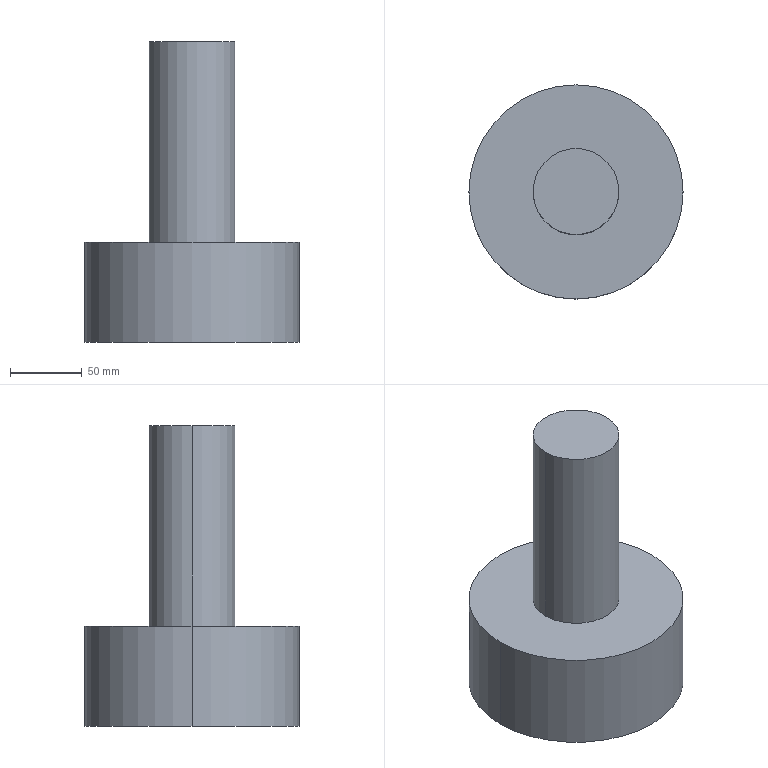Part | SolidWorks | features ICE 2, Extrusion 1 | 1 solid | 10 faces | box 149.5 x 149.5 x 210 mm | volume 1568199 mm3 | cylinder 6 | plane 4 | commonest cylinder face diameters 32.5 x2 60 x2 149.5 x2
STEP:
#1=CARTESIAN_POINT('',(30.,0.,210.));
#2=VERTEX_POINT('',#1);
#3=CARTESIAN_POINT('',(-30.,0.,210.));
#4=VERTEX_POINT('',#3);
#5=CARTESIAN_POINT('',(0.,0.,210.));
#6=DIRECTION('',(0.,0.,1.));
#7=DIRECTION('',(1.,0.,0.));
#8=AXIS2_PLACEMENT_3D('',#5,#6,#7);
#9=CIRCLE('',#8,30.);
#10=EDGE_CURVE('',#2,#4,#9,.T.);
#11=ORIENTED_EDGE('',*,*,#10,.F.);
#12=CARTESIAN_POINT('',(30.,0.,70.));
#13=VERTEX_POINT('',#12);
#14=CARTESIAN_POINT('',(30.,0.,210.));
#15=DIRECTION('',(0.,0.,-1.));
#16=VECTOR('',#15,1000.);
#17=LINE('',#14,#16);
#18=EDGE_CURVE('',#2,#13,#17,.T.);
#19=ORIENTED_EDGE('',*,*,#18,.T.);
#20=CARTESIAN_POINT('',(-30.,0.,70.));
#21=VERTEX_POINT('',#20);
#22=CARTESIAN_POINT('',(0.,0.,70.));
#23=DIRECTION('',(0.,0.,1.));
#24=DIRECTION('',(1.,0.,0.));
#25=AXIS2_PLACEMENT_3D('',#22,#23,#24);
#26=CIRCLE('',#25,30.);
#27=EDGE_CURVE('',#13,#21,#26,.T.);
#28=ORIENTED_EDGE('',*,*,#27,.T.);
#29=CARTESIAN_POINT('',(-30.,0.,210.));
#30=DIRECTION('',(0.,0.,-1.));
#31=VECTOR('',#30,1000.);
#32=LINE('',#29,#31);
#33=EDGE_CURVE('',#4,#21,#32,.T.);
#34=ORIENTED_EDGE('',*,*,#33,.F.);
#35=EDGE_LOOP('',(#11,#19,#28,#34));
#36=FACE_OUTER_BOUND('',#35,.T.);
#37=CARTESIAN_POINT('',(0.,0.,210.));
#38=DIRECTION('',(0.,0.,-1.));
#39=DIRECTION('',(-1.,0.,0.));
#40=AXIS2_PLACEMENT_3D('',#37,#38,#39);
#41=CYLINDRICAL_SURFACE('',#40,30.);
#42=ADVANCED_FACE('',(#36),#41,.T.);
#43=CARTESIAN_POINT('',(16.25,0.,68.));
#44=VERTEX_POINT('',#43);
#45=CARTESIAN_POINT('',(-16.25,0.,68.));
#46=VERTEX_POINT('',#45);
#47=CARTESIAN_POINT('',(0.,0.,68.));
#48=DIRECTION('',(0.,0.,-1.));
#49=DIRECTION('',(-1.,0.,0.));
#50=AXIS2_PLACEMENT_3D('',#47,#48,#49);
#51=CIRCLE('',#50,16.25);
#52=EDGE_CURVE('',#44,#46,#51,.T.);
#53=ORIENTED_EDGE('',*,*,#52,.F.);
#54=CARTESIAN_POINT('',(16.25,0.,0.));
#55=VERTEX_POINT('',#54);
#56=CARTESIAN_POINT('',(16.25,0.,68.));
#57=DIRECTION('',(0.,0.,-1.));
#58=VECTOR('',#57,1000.);
#59=LINE('',#56,#58);
#60=EDGE_CURVE('',#44,#55,#59,.T.);
#61=ORIENTED_EDGE('',*,*,#60,.T.);
#62=CARTESIAN_POINT('',(-16.25,0.,0.));
#63=VERTEX_POINT('',#62);
#64=CARTESIAN_POINT('',(0.,0.,0.));
#65=DIRECTION('',(0.,0.,-1.));
#66=DIRECTION('',(-1.,0.,0.));
#67=AXIS2_PLACEMENT_3D('',#64,#65,#66);
#68=CIRCLE('',#67,16.25);
#69=EDGE_CURVE('',#55,#63,#68,.T.);
#70=ORIENTED_EDGE('',*,*,#69,.T.);
#71=CARTESIAN_POINT('',(-16.25,0.,68.));
#72=DIRECTION('',(0.,0.,-1.));
#73=VECTOR('',#72,1000.);
#74=LINE('',#71,#73);
#75=EDGE_CURVE('',#46,#63,#74,.T.);
#76=ORIENTED_EDGE('',*,*,#75,.F.);
#77=EDGE_LOOP('',(#53,#61,#70,#76));
#78=FACE_OUTER_BOUND('',#77,.T.);
#79=CARTESIAN_POINT('',(0.,0.,68.));
#80=DIRECTION('',(0.,0.,-1.));
#81=DIRECTION('',(-1.,0.,0.));
#82=AXIS2_PLACEMENT_3D('',#79,#80,#81);
#83=CYLINDRICAL_SURFACE('',#82,16.25);
#84=ADVANCED_FACE('',(#78),#83,.F.);
#85=CARTESIAN_POINT('',(74.75,0.,70.));
#86=VERTEX_POINT('',#85);
#87=CARTESIAN_POINT('',(-74.75,0.,70.));
#88=VERTEX_POINT('',#87);
#89=CARTESIAN_POINT('',(0.,0.,70.));
#90=DIRECTION('',(0.,0.,1.));
#91=DIRECTION('',(1.,0.,0.));
#92=AXIS2_PLACEMENT_3D('',#89,#90,#91);
#93=CIRCLE('',#92,74.75);
#94=EDGE_CURVE('',#86,#88,#93,.T.);
#95=ORIENTED_EDGE('',*,*,#94,.F.);
#96=CARTESIAN_POINT('',(74.75,0.,0.));
#97=VERTEX_POINT('',#96);
#98=CARTESIAN_POINT('',(74.75,0.,70.));
#99=DIRECTION('',(0.,0.,-1.));
#100=VECTOR('',#99,1000.);
#101=LINE('',#98,#100);
#102=EDGE_CURVE('',#86,#97,#101,.T.);
#103=ORIENTED_EDGE('',*,*,#102,.T.);
#104=CARTESIAN_POINT('',(-74.75,0.,0.));
#105=VERTEX_POINT('',#104);
#106=CARTESIAN_POINT('',(0.,0.,0.));
#107=DIRECTION('',(0.,0.,1.));
#108=DIRECTION('',(1.,0.,0.));
#109=AXIS2_PLACEMENT_3D('',#106,#107,#108);
#110=CIRCLE('',#109,74.75);
#111=EDGE_CURVE('',#97,#105,#110,.T.);
#112=ORIENTED_EDGE('',*,*,#111,.T.);
#113=CARTESIAN_POINT('',(-74.75,0.,70.));
#114=DIRECTION('',(0.,0.,-1.));
#115=VECTOR('',#114,1000.);
#116=LINE('',#113,#115);
#117=EDGE_CURVE('',#88,#105,#116,.T.);
#118=ORIENTED_EDGE('',*,*,#117,.F.);
#119=EDGE_LOOP('',(#95,#103,#112,#118));
#120=FACE_OUTER_BOUND('',#119,.T.);
#121=CARTESIAN_POINT('',(0.,0.,70.));
#122=DIRECTION('',(0.,0.,-1.));
#123=DIRECTION('',(-1.,0.,0.));
#124=AXIS2_PLACEMENT_3D('',#121,#122,#123);
#125=CYLINDRICAL_SURFACE('',#124,74.75);
#126=ADVANCED_FACE('',(#120),#125,.T.);
#127=ORIENTED_EDGE('',*,*,#102,.F.);
#128=CARTESIAN_POINT('',(0.,0.,70.));
#129=DIRECTION('',(0.,0.,1.));
#130=DIRECTION('',(1.,0.,0.));
#131=AXIS2_PLACEMENT_3D('',#128,#129,#130);
#132=CIRCLE('',#131,74.75);
#133=EDGE_CURVE('',#88,#86,#132,.T.);
#134=ORIENTED_EDGE('',*,*,#133,.F.);
#135=ORIENTED_EDGE('',*,*,#117,.T.);
#136=CARTESIAN_POINT('',(0.,0.,0.));
#137=DIRECTION('',(0.,0.,1.));
#138=DIRECTION('',(1.,0.,0.));
#139=AXIS2_PLACEMENT_3D('',#136,#137,#138);
#140=CIRCLE('',#139,74.75);
#141=EDGE_CURVE('',#105,#97,#140,.T.);
#142=ORIENTED_EDGE('',*,*,#141,.T.);
#143=EDGE_LOOP('',(#127,#134,#135,#142));
#144=FACE_OUTER_BOUND('',#143,.T.);
#145=CARTESIAN_POINT('',(0.,0.,70.));
#146=DIRECTION('',(0.,0.,-1.));
#147=DIRECTION('',(-1.,0.,0.));
#148=AXIS2_PLACEMENT_3D('',#145,#146,#147);
#149=CYLINDRICAL_SURFACE('',#148,74.75);
#150=ADVANCED_FACE('',(#144),#149,.T.);
#151=CARTESIAN_POINT('',(0.,0.,70.));
#152=DIRECTION('',(0.,0.,1.));
#153=DIRECTION('',(1.,0.,0.));
#154=AXIS2_PLACEMENT_3D('',#151,#152,#153);
#155=CIRCLE('',#154,30.);
#156=EDGE_CURVE('',#21,#13,#155,.T.);
#157=ORIENTED_EDGE('',*,*,#156,.F.);
#158=ORIENTED_EDGE('',*,*,#27,.F.);
#159=EDGE_LOOP('',(#157,#158));
#160=FACE_BOUND('',#159,.T.);
#161=ORIENTED_EDGE('',*,*,#133,.T.);
#162=ORIENTED_EDGE('',*,*,#94,.T.);
#163=EDGE_LOOP('',(#161,#162));
#164=FACE_OUTER_BOUND('',#163,.T.);
#165=CARTESIAN_POINT('',(0.,0.,70.));
#166=DIRECTION('',(0.,0.,1.));
#167=DIRECTION('',(1.,0.,0.));
#168=AXIS2_PLACEMENT_3D('',#165,#166,#167);
#169=PLANE('',#168);
#170=ADVANCED_FACE('',(#160,#164),#169,.T.);
#171=CARTESIAN_POINT('',(0.,0.,0.));
#172=DIRECTION('',(0.,0.,-1.));
#173=DIRECTION('',(-1.,0.,0.));
#174=AXIS2_PLACEMENT_3D('',#171,#172,#173);
#175=CIRCLE('',#174,16.25);
#176=EDGE_CURVE('',#63,#55,#175,.T.);
#177=ORIENTED_EDGE('',*,*,#176,.F.);
#178=ORIENTED_EDGE('',*,*,#69,.F.);
#179=EDGE_LOOP('',(#177,#178));
#180=FACE_BOUND('',#179,.T.);
#181=ORIENTED_EDGE('',*,*,#141,.F.);
#182=ORIENTED_EDGE('',*,*,#111,.F.);
#183=EDGE_LOOP('',(#181,#182));
#184=FACE_OUTER_BOUND('',#183,.T.);
#185=CARTESIAN_POINT('',(0.,0.,0.));
#186=DIRECTION('',(0.,0.,1.));
#187=DIRECTION('',(1.,0.,0.));
#188=AXIS2_PLACEMENT_3D('',#185,#186,#187);
#189=PLANE('',#188);
#190=ADVANCED_FACE('',(#180,#184),#189,.F.);
#191=ORIENTED_EDGE('',*,*,#60,.F.);
#192=CARTESIAN_POINT('',(0.,0.,68.));
#193=DIRECTION('',(0.,0.,-1.));
#194=DIRECTION('',(-1.,0.,0.));
#195=AXIS2_PLACEMENT_3D('',#192,#193,#194);
#196=CIRCLE('',#195,16.25);
#197=EDGE_CURVE('',#46,#44,#196,.T.);
#198=ORIENTED_EDGE('',*,*,#197,.F.);
#199=ORIENTED_EDGE('',*,*,#75,.T.);
#200=ORIENTED_EDGE('',*,*,#176,.T.);
#201=EDGE_LOOP('',(#191,#198,#199,#200));
#202=FACE_OUTER_BOUND('',#201,.T.);
#203=CARTESIAN_POINT('',(0.,0.,68.));
#204=DIRECTION('',(0.,0.,-1.));
#205=DIRECTION('',(-1.,0.,0.));
#206=AXIS2_PLACEMENT_3D('',#203,#204,#205);
#207=CYLINDRICAL_SURFACE('',#206,16.25);
#208=ADVANCED_FACE('',(#202),#207,.F.);
#209=ORIENTED_EDGE('',*,*,#197,.T.);
#210=ORIENTED_EDGE('',*,*,#52,.T.);
#211=EDGE_LOOP('',(#209,#210));
#212=FACE_OUTER_BOUND('',#211,.T.);
#213=CARTESIAN_POINT('',(0.,0.,68.));
#214=DIRECTION('',(0.,0.,-1.));
#215=DIRECTION('',(-1.,0.,0.));
#216=AXIS2_PLACEMENT_3D('',#213,#214,#215);
#217=PLANE('',#216);
#218=ADVANCED_FACE('',(#212),#217,.T.);
#219=ORIENTED_EDGE('',*,*,#18,.F.);
#220=CARTESIAN_POINT('',(0.,0.,210.));
#221=DIRECTION('',(0.,0.,1.));
#222=DIRECTION('',(1.,0.,0.));
#223=AXIS2_PLACEMENT_3D('',#220,#221,#222);
#224=CIRCLE('',#223,30.);
#225=EDGE_CURVE('',#4,#2,#224,.T.);
#226=ORIENTED_EDGE('',*,*,#225,.F.);
#227=ORIENTED_EDGE('',*,*,#33,.T.);
#228=ORIENTED_EDGE('',*,*,#156,.T.);
#229=EDGE_LOOP('',(#219,#226,#227,#228));
#230=FACE_OUTER_BOUND('',#229,.T.);
#231=CARTESIAN_POINT('',(0.,0.,210.));
#232=DIRECTION('',(0.,0.,-1.));
#233=DIRECTION('',(-1.,0.,0.));
#234=AXIS2_PLACEMENT_3D('',#231,#232,#233);
#235=CYLINDRICAL_SURFACE('',#234,30.);
#236=ADVANCED_FACE('',(#230),#235,.T.);
#237=ORIENTED_EDGE('',*,*,#225,.T.);
#238=ORIENTED_EDGE('',*,*,#10,.T.);
#239=EDGE_LOOP('',(#237,#238));
#240=FACE_OUTER_BOUND('',#239,.T.);
#241=CARTESIAN_POINT('',(0.,0.,210.));
#242=DIRECTION('',(0.,0.,1.));
#243=DIRECTION('',(1.,0.,0.));
#244=AXIS2_PLACEMENT_3D('',#241,#242,#243);
#245=PLANE('',#244);
#246=ADVANCED_FACE('',(#240),#245,.T.);
#247=CLOSED_SHELL('',(#42,#84,#126,#150,#170,#190,#208,#218,#236,#246));
#248=MANIFOLD_SOLID_BREP('',#247);
#249=CARTESIAN_POINT('',(0.,0.,0.));
#250=DIRECTION('',(0.,0.,1.));
#251=DIRECTION('',(1.,0.,0.));
#252=AXIS2_PLACEMENT_3D('',#249,#250,#251);
#253=(LENGTH_UNIT()NAMED_UNIT(*)SI_UNIT(.MILLI.,.METRE.));
#254=UNCERTAINTY_MEASURE_WITH_UNIT(LENGTH_MEASURE(0.00001),#253,'','');
#255=(NAMED_UNIT(*)PLANE_ANGLE_UNIT()SI_UNIT($,.RADIAN.));
#256=(NAMED_UNIT(*)SI_UNIT($,.STERADIAN.)SOLID_ANGLE_UNIT());
#257=(GEOMETRIC_REPRESENTATION_CONTEXT(3)GLOBAL_UNCERTAINTY_ASSIGNED_CONTEXT((#254))GLOBAL_UNIT_ASSIGNED_CONTEXT((#253,#255,#256))REPRESENTATION_CONTEXT('',''));
#258=ADVANCED_BREP_SHAPE_REPRESENTATION('',(#248,#252),#257);